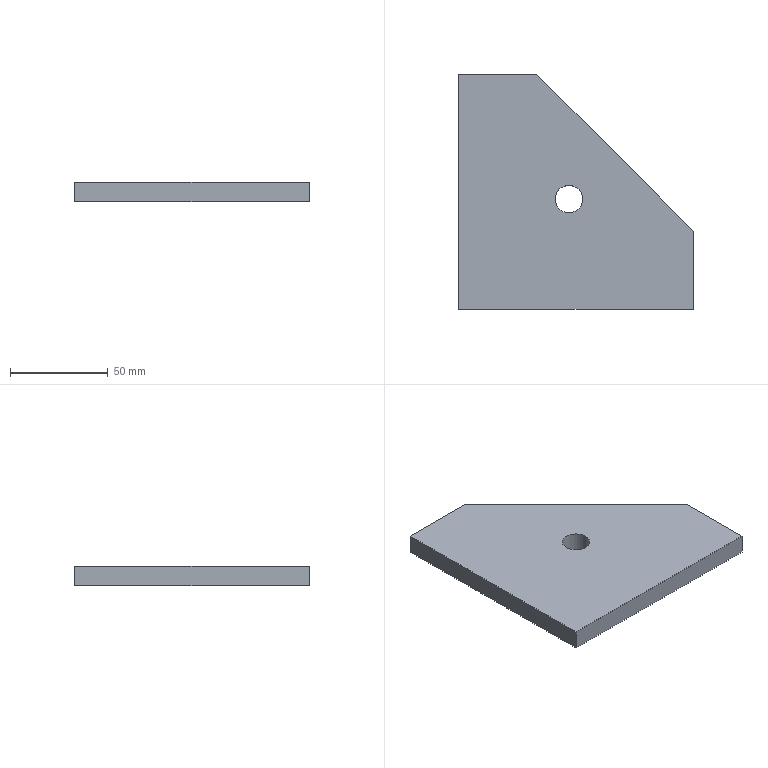Part | SolidWorks | features Extrusion 1, HoleWzd 1 | 1 solid | 9 faces | box 120 x 120 x 10 mm | volume 110461 mm3 | plane 7 | cylinder 2 | commonest cylinder face diameters 14 x2
STEP:
#1=CARTESIAN_POINT('',(63.38,56.38,10.));
#2=VERTEX_POINT('',#1);
#3=CARTESIAN_POINT('',(49.38,56.38,10.));
#4=VERTEX_POINT('',#3);
#5=CARTESIAN_POINT('',(56.38,56.38,10.));
#6=DIRECTION('',(0.,0.,-1.));
#7=DIRECTION('',(-1.,0.,0.));
#8=AXIS2_PLACEMENT_3D('',#5,#6,#7);
#9=CIRCLE('',#8,7.);
#10=EDGE_CURVE('',#2,#4,#9,.T.);
#11=ORIENTED_EDGE('',*,*,#10,.F.);
#12=CARTESIAN_POINT('',(63.38,56.38,0.));
#13=VERTEX_POINT('',#12);
#14=CARTESIAN_POINT('',(63.38,56.38,0.));
#15=DIRECTION('',(0.,0.,-1.));
#16=VECTOR('',#15,1000.);
#17=LINE('',#14,#16);
#18=EDGE_CURVE('',#2,#13,#17,.T.);
#19=ORIENTED_EDGE('',*,*,#18,.T.);
#20=CARTESIAN_POINT('',(49.38,56.38,0.));
#21=VERTEX_POINT('',#20);
#22=CARTESIAN_POINT('',(56.38,56.38,0.));
#23=DIRECTION('',(0.,0.,-1.));
#24=DIRECTION('',(-1.,0.,0.));
#25=AXIS2_PLACEMENT_3D('',#22,#23,#24);
#26=CIRCLE('',#25,7.);
#27=EDGE_CURVE('',#13,#21,#26,.T.);
#28=ORIENTED_EDGE('',*,*,#27,.T.);
#29=CARTESIAN_POINT('',(49.38,56.38,0.));
#30=DIRECTION('',(0.,0.,-1.));
#31=VECTOR('',#30,1000.);
#32=LINE('',#29,#31);
#33=EDGE_CURVE('',#4,#21,#32,.T.);
#34=ORIENTED_EDGE('',*,*,#33,.F.);
#35=EDGE_LOOP('',(#11,#19,#28,#34));
#36=FACE_OUTER_BOUND('',#35,.T.);
#37=CARTESIAN_POINT('',(56.38,56.38,0.));
#38=DIRECTION('',(0.,0.,-1.));
#39=DIRECTION('',(-1.,0.,0.));
#40=AXIS2_PLACEMENT_3D('',#37,#38,#39);
#41=CYLINDRICAL_SURFACE('',#40,7.);
#42=ADVANCED_FACE('',(#36),#41,.F.);
#43=CARTESIAN_POINT('',(40.,120.,0.));
#44=VERTEX_POINT('',#43);
#45=CARTESIAN_POINT('',(0.,120.,0.));
#46=VERTEX_POINT('',#45);
#47=CARTESIAN_POINT('',(40.,120.,0.));
#48=DIRECTION('',(-1.,0.,0.));
#49=VECTOR('',#48,1000.);
#50=LINE('',#47,#49);
#51=EDGE_CURVE('',#44,#46,#50,.T.);
#52=ORIENTED_EDGE('',*,*,#51,.T.);
#53=CARTESIAN_POINT('',(0.,120.,10.));
#54=VERTEX_POINT('',#53);
#55=CARTESIAN_POINT('',(0.,120.,10.));
#56=DIRECTION('',(0.,0.,-1.));
#57=VECTOR('',#56,1000.);
#58=LINE('',#55,#57);
#59=EDGE_CURVE('',#54,#46,#58,.T.);
#60=ORIENTED_EDGE('',*,*,#59,.F.);
#61=CARTESIAN_POINT('',(40.,120.,10.));
#62=VERTEX_POINT('',#61);
#63=CARTESIAN_POINT('',(40.,120.,10.));
#64=DIRECTION('',(-1.,0.,0.));
#65=VECTOR('',#64,1000.);
#66=LINE('',#63,#65);
#67=EDGE_CURVE('',#62,#54,#66,.T.);
#68=ORIENTED_EDGE('',*,*,#67,.F.);
#69=CARTESIAN_POINT('',(40.,120.,10.));
#70=DIRECTION('',(0.,0.,-1.));
#71=VECTOR('',#70,1000.);
#72=LINE('',#69,#71);
#73=EDGE_CURVE('',#62,#44,#72,.T.);
#74=ORIENTED_EDGE('',*,*,#73,.T.);
#75=EDGE_LOOP('',(#52,#60,#68,#74));
#76=FACE_OUTER_BOUND('',#75,.T.);
#77=CARTESIAN_POINT('',(40.,120.,10.));
#78=DIRECTION('',(0.,-1.,0.));
#79=DIRECTION('',(0.,0.,-1.));
#80=AXIS2_PLACEMENT_3D('',#77,#78,#79);
#81=PLANE('',#80);
#82=ADVANCED_FACE('',(#76),#81,.F.);
#83=CARTESIAN_POINT('',(0.,0.,0.));
#84=VERTEX_POINT('',#83);
#85=CARTESIAN_POINT('',(0.,120.,0.));
#86=DIRECTION('',(0.,-1.,0.));
#87=VECTOR('',#86,1000.);
#88=LINE('',#85,#87);
#89=EDGE_CURVE('',#46,#84,#88,.T.);
#90=ORIENTED_EDGE('',*,*,#89,.T.);
#91=CARTESIAN_POINT('',(0.,0.,10.));
#92=VERTEX_POINT('',#91);
#93=CARTESIAN_POINT('',(0.,0.,10.));
#94=DIRECTION('',(0.,0.,-1.));
#95=VECTOR('',#94,1000.);
#96=LINE('',#93,#95);
#97=EDGE_CURVE('',#92,#84,#96,.T.);
#98=ORIENTED_EDGE('',*,*,#97,.F.);
#99=CARTESIAN_POINT('',(0.,120.,10.));
#100=DIRECTION('',(0.,-1.,0.));
#101=VECTOR('',#100,1000.);
#102=LINE('',#99,#101);
#103=EDGE_CURVE('',#54,#92,#102,.T.);
#104=ORIENTED_EDGE('',*,*,#103,.F.);
#105=ORIENTED_EDGE('',*,*,#59,.T.);
#106=EDGE_LOOP('',(#90,#98,#104,#105));
#107=FACE_OUTER_BOUND('',#106,.T.);
#108=CARTESIAN_POINT('',(0.,120.,10.));
#109=DIRECTION('',(1.,0.,0.));
#110=DIRECTION('',(0.,0.,-1.));
#111=AXIS2_PLACEMENT_3D('',#108,#109,#110);
#112=PLANE('',#111);
#113=ADVANCED_FACE('',(#107),#112,.F.);
#114=CARTESIAN_POINT('',(120.,0.,0.));
#115=VERTEX_POINT('',#114);
#116=CARTESIAN_POINT('',(0.,0.,0.));
#117=DIRECTION('',(1.,0.,0.));
#118=VECTOR('',#117,1000.);
#119=LINE('',#116,#118);
#120=EDGE_CURVE('',#84,#115,#119,.T.);
#121=ORIENTED_EDGE('',*,*,#120,.T.);
#122=CARTESIAN_POINT('',(120.,0.,10.));
#123=VERTEX_POINT('',#122);
#124=CARTESIAN_POINT('',(120.,0.,10.));
#125=DIRECTION('',(0.,0.,-1.));
#126=VECTOR('',#125,1000.);
#127=LINE('',#124,#126);
#128=EDGE_CURVE('',#123,#115,#127,.T.);
#129=ORIENTED_EDGE('',*,*,#128,.F.);
#130=CARTESIAN_POINT('',(0.,0.,10.));
#131=DIRECTION('',(1.,0.,0.));
#132=VECTOR('',#131,1000.);
#133=LINE('',#130,#132);
#134=EDGE_CURVE('',#92,#123,#133,.T.);
#135=ORIENTED_EDGE('',*,*,#134,.F.);
#136=ORIENTED_EDGE('',*,*,#97,.T.);
#137=EDGE_LOOP('',(#121,#129,#135,#136));
#138=FACE_OUTER_BOUND('',#137,.T.);
#139=CARTESIAN_POINT('',(0.,0.,10.));
#140=DIRECTION('',(0.,1.,0.));
#141=DIRECTION('',(0.,0.,1.));
#142=AXIS2_PLACEMENT_3D('',#139,#140,#141);
#143=PLANE('',#142);
#144=ADVANCED_FACE('',(#138),#143,.F.);
#145=CARTESIAN_POINT('',(120.,40.,0.));
#146=VERTEX_POINT('',#145);
#147=CARTESIAN_POINT('',(120.,0.,0.));
#148=DIRECTION('',(0.,1.,0.));
#149=VECTOR('',#148,1000.);
#150=LINE('',#147,#149);
#151=EDGE_CURVE('',#115,#146,#150,.T.);
#152=ORIENTED_EDGE('',*,*,#151,.T.);
#153=CARTESIAN_POINT('',(120.,40.,10.));
#154=VERTEX_POINT('',#153);
#155=CARTESIAN_POINT('',(120.,40.,10.));
#156=DIRECTION('',(0.,0.,-1.));
#157=VECTOR('',#156,1000.);
#158=LINE('',#155,#157);
#159=EDGE_CURVE('',#154,#146,#158,.T.);
#160=ORIENTED_EDGE('',*,*,#159,.F.);
#161=CARTESIAN_POINT('',(120.,0.,10.));
#162=DIRECTION('',(0.,1.,0.));
#163=VECTOR('',#162,1000.);
#164=LINE('',#161,#163);
#165=EDGE_CURVE('',#123,#154,#164,.T.);
#166=ORIENTED_EDGE('',*,*,#165,.F.);
#167=ORIENTED_EDGE('',*,*,#128,.T.);
#168=EDGE_LOOP('',(#152,#160,#166,#167));
#169=FACE_OUTER_BOUND('',#168,.T.);
#170=CARTESIAN_POINT('',(120.,0.,10.));
#171=DIRECTION('',(-1.,0.,0.));
#172=DIRECTION('',(0.,0.,1.));
#173=AXIS2_PLACEMENT_3D('',#170,#171,#172);
#174=PLANE('',#173);
#175=ADVANCED_FACE('',(#169),#174,.F.);
#176=CARTESIAN_POINT('',(120.,40.,0.));
#177=DIRECTION('',(-0.7071,0.7071,0.));
#178=VECTOR('',#177,1000.);
#179=LINE('',#176,#178);
#180=EDGE_CURVE('',#146,#44,#179,.T.);
#181=ORIENTED_EDGE('',*,*,#180,.T.);
#182=ORIENTED_EDGE('',*,*,#73,.F.);
#183=CARTESIAN_POINT('',(120.,40.,10.));
#184=DIRECTION('',(-0.7071,0.7071,0.));
#185=VECTOR('',#184,1000.);
#186=LINE('',#183,#185);
#187=EDGE_CURVE('',#154,#62,#186,.T.);
#188=ORIENTED_EDGE('',*,*,#187,.F.);
#189=ORIENTED_EDGE('',*,*,#159,.T.);
#190=EDGE_LOOP('',(#181,#182,#188,#189));
#191=FACE_OUTER_BOUND('',#190,.T.);
#192=CARTESIAN_POINT('',(120.,40.,10.));
#193=DIRECTION('',(-0.7071,-0.7071,0.));
#194=DIRECTION('',(0.7071,-0.7071,0.));
#195=AXIS2_PLACEMENT_3D('',#192,#193,#194);
#196=PLANE('',#195);
#197=ADVANCED_FACE('',(#191),#196,.F.);
#198=CARTESIAN_POINT('',(56.38,56.38,10.));
#199=DIRECTION('',(0.,0.,-1.));
#200=DIRECTION('',(-1.,0.,0.));
#201=AXIS2_PLACEMENT_3D('',#198,#199,#200);
#202=CIRCLE('',#201,7.);
#203=EDGE_CURVE('',#4,#2,#202,.T.);
#204=ORIENTED_EDGE('',*,*,#203,.T.);
#205=ORIENTED_EDGE('',*,*,#10,.T.);
#206=EDGE_LOOP('',(#204,#205));
#207=FACE_BOUND('',#206,.T.);
#208=ORIENTED_EDGE('',*,*,#67,.T.);
#209=ORIENTED_EDGE('',*,*,#103,.T.);
#210=ORIENTED_EDGE('',*,*,#134,.T.);
#211=ORIENTED_EDGE('',*,*,#165,.T.);
#212=ORIENTED_EDGE('',*,*,#187,.T.);
#213=EDGE_LOOP('',(#208,#209,#210,#211,#212));
#214=FACE_OUTER_BOUND('',#213,.T.);
#215=CARTESIAN_POINT('',(0.,0.,10.));
#216=DIRECTION('',(0.,0.,1.));
#217=DIRECTION('',(1.,0.,0.));
#218=AXIS2_PLACEMENT_3D('',#215,#216,#217);
#219=PLANE('',#218);
#220=ADVANCED_FACE('',(#207,#214),#219,.T.);
#221=CARTESIAN_POINT('',(56.38,56.38,0.));
#222=DIRECTION('',(0.,0.,-1.));
#223=DIRECTION('',(-1.,0.,0.));
#224=AXIS2_PLACEMENT_3D('',#221,#222,#223);
#225=CIRCLE('',#224,7.);
#226=EDGE_CURVE('',#21,#13,#225,.T.);
#227=ORIENTED_EDGE('',*,*,#226,.F.);
#228=ORIENTED_EDGE('',*,*,#27,.F.);
#229=EDGE_LOOP('',(#227,#228));
#230=FACE_BOUND('',#229,.T.);
#231=ORIENTED_EDGE('',*,*,#51,.F.);
#232=ORIENTED_EDGE('',*,*,#180,.F.);
#233=ORIENTED_EDGE('',*,*,#151,.F.);
#234=ORIENTED_EDGE('',*,*,#120,.F.);
#235=ORIENTED_EDGE('',*,*,#89,.F.);
#236=EDGE_LOOP('',(#231,#232,#233,#234,#235));
#237=FACE_OUTER_BOUND('',#236,.T.);
#238=CARTESIAN_POINT('',(0.,0.,0.));
#239=DIRECTION('',(0.,0.,1.));
#240=DIRECTION('',(1.,0.,0.));
#241=AXIS2_PLACEMENT_3D('',#238,#239,#240);
#242=PLANE('',#241);
#243=ADVANCED_FACE('',(#230,#237),#242,.F.);
#244=ORIENTED_EDGE('',*,*,#18,.F.);
#245=ORIENTED_EDGE('',*,*,#203,.F.);
#246=ORIENTED_EDGE('',*,*,#33,.T.);
#247=ORIENTED_EDGE('',*,*,#226,.T.);
#248=EDGE_LOOP('',(#244,#245,#246,#247));
#249=FACE_OUTER_BOUND('',#248,.T.);
#250=CARTESIAN_POINT('',(56.38,56.38,0.));
#251=DIRECTION('',(0.,0.,-1.));
#252=DIRECTION('',(-1.,0.,0.));
#253=AXIS2_PLACEMENT_3D('',#250,#251,#252);
#254=CYLINDRICAL_SURFACE('',#253,7.);
#255=ADVANCED_FACE('',(#249),#254,.F.);
#256=CLOSED_SHELL('',(#42,#82,#113,#144,#175,#197,#220,#243,#255));
#257=MANIFOLD_SOLID_BREP('',#256);
#258=CARTESIAN_POINT('',(0.,0.,0.));
#259=DIRECTION('',(0.,0.,1.));
#260=DIRECTION('',(1.,0.,0.));
#261=AXIS2_PLACEMENT_3D('',#258,#259,#260);
#262=(LENGTH_UNIT()NAMED_UNIT(*)SI_UNIT(.MILLI.,.METRE.));
#263=UNCERTAINTY_MEASURE_WITH_UNIT(LENGTH_MEASURE(0.00001),#262,'','');
#264=(NAMED_UNIT(*)PLANE_ANGLE_UNIT()SI_UNIT($,.RADIAN.));
#265=(NAMED_UNIT(*)SI_UNIT($,.STERADIAN.)SOLID_ANGLE_UNIT());
#266=(GEOMETRIC_REPRESENTATION_CONTEXT(3)GLOBAL_UNCERTAINTY_ASSIGNED_CONTEXT((#263))GLOBAL_UNIT_ASSIGNED_CONTEXT((#262,#264,#265))REPRESENTATION_CONTEXT('',''));
#267=ADVANCED_BREP_SHAPE_REPRESENTATION('',(#257,#261),#266);